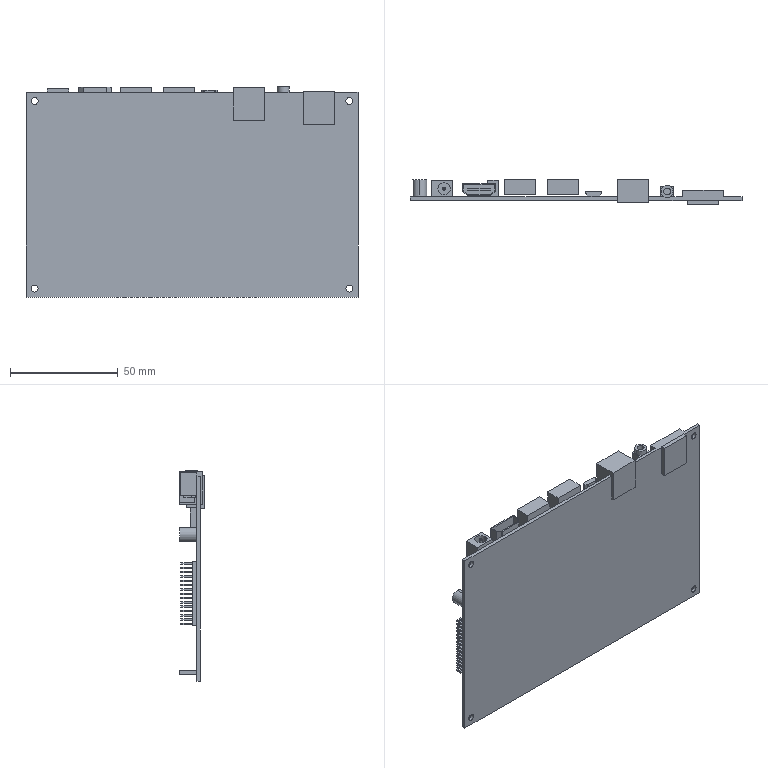Part | SolidWorks | features BaseBody 5 | 5 solids | 270 faces | box 154 x 11.8 x 97.6 mm | volume 32495 mm3 | plane 244 | cylinder 24 | spline 2 | commonest cylinder face diameters 3.2 x10 1 x4 1.5 x2 2 x2 5.5 x2 5.7 x2